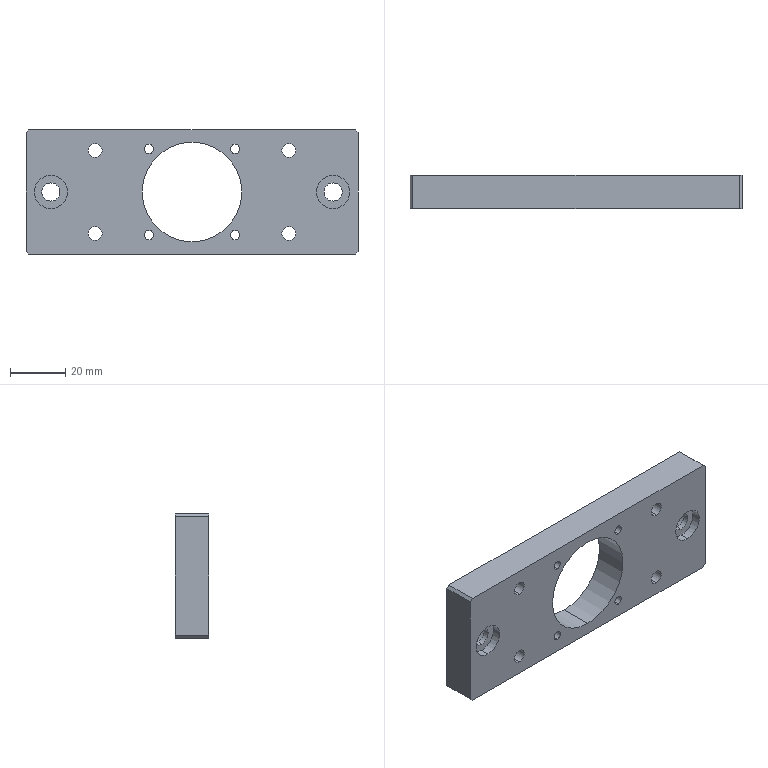Part | SolidWorks | features HoleWzd 4, ICE 2, Chamfer 1, Extrusion 1 | 1 solid | 48 faces | box 120 x 12 x 45 mm | volume 48954 mm3 | cylinder 32 | plane 14 | cone 2 | commonest cylinder face diameters 3.3 x10 5 x8 6.6 x4 11 x4 12 x4 36 x2
STEP:
#1=CARTESIAN_POINT('',(35.,0.,17.5));
#2=VERTEX_POINT('',#1);
#3=CARTESIAN_POINT('',(35.,0.,12.5));
#4=VERTEX_POINT('',#3);
#5=CARTESIAN_POINT('',(35.,0.,15.));
#6=DIRECTION('',(0.,-1.,0.));
#7=DIRECTION('',(0.,0.,-1.));
#8=AXIS2_PLACEMENT_3D('',#5,#6,#7);
#9=CIRCLE('',#8,2.5);
#10=EDGE_CURVE('',#2,#4,#9,.T.);
#11=ORIENTED_EDGE('',*,*,#10,.T.);
#12=CARTESIAN_POINT('',(35.,12.,12.5));
#13=VERTEX_POINT('',#12);
#14=CARTESIAN_POINT('',(35.,12.,12.5));
#15=DIRECTION('',(0.,1.,0.));
#16=VECTOR('',#15,1000.);
#17=LINE('',#14,#16);
#18=EDGE_CURVE('',#4,#13,#17,.T.);
#19=ORIENTED_EDGE('',*,*,#18,.T.);
#20=CARTESIAN_POINT('',(35.,12.,17.5));
#21=VERTEX_POINT('',#20);
#22=CARTESIAN_POINT('',(35.,12.,15.));
#23=DIRECTION('',(0.,1.,0.));
#24=DIRECTION('',(0.,0.,1.));
#25=AXIS2_PLACEMENT_3D('',#22,#23,#24);
#26=CIRCLE('',#25,2.5);
#27=EDGE_CURVE('',#13,#21,#26,.T.);
#28=ORIENTED_EDGE('',*,*,#27,.T.);
#29=CARTESIAN_POINT('',(35.,12.,17.5));
#30=DIRECTION('',(0.,1.,0.));
#31=VECTOR('',#30,1000.);
#32=LINE('',#29,#31);
#33=EDGE_CURVE('',#2,#21,#32,.T.);
#34=ORIENTED_EDGE('',*,*,#33,.F.);
#35=EDGE_LOOP('',(#11,#19,#28,#34));
#36=FACE_OUTER_BOUND('',#35,.T.);
#37=CARTESIAN_POINT('',(35.,12.,15.));
#38=DIRECTION('',(0.,1.,0.));
#39=DIRECTION('',(0.,0.,1.));
#40=AXIS2_PLACEMENT_3D('',#37,#38,#39);
#41=CYLINDRICAL_SURFACE('',#40,2.5);
#42=ADVANCED_FACE('',(#36),#41,.F.);
#43=CARTESIAN_POINT('',(35.,0.,-12.5));
#44=VERTEX_POINT('',#43);
#45=CARTESIAN_POINT('',(35.,0.,-17.5));
#46=VERTEX_POINT('',#45);
#47=CARTESIAN_POINT('',(35.,0.,-15.));
#48=DIRECTION('',(0.,-1.,0.));
#49=DIRECTION('',(0.,0.,-1.));
#50=AXIS2_PLACEMENT_3D('',#47,#48,#49);
#51=CIRCLE('',#50,2.5);
#52=EDGE_CURVE('',#44,#46,#51,.T.);
#53=ORIENTED_EDGE('',*,*,#52,.T.);
#54=CARTESIAN_POINT('',(35.,12.,-17.5));
#55=VERTEX_POINT('',#54);
#56=CARTESIAN_POINT('',(35.,12.,-17.5));
#57=DIRECTION('',(0.,1.,0.));
#58=VECTOR('',#57,1000.);
#59=LINE('',#56,#58);
#60=EDGE_CURVE('',#46,#55,#59,.T.);
#61=ORIENTED_EDGE('',*,*,#60,.T.);
#62=CARTESIAN_POINT('',(35.,12.,-12.5));
#63=VERTEX_POINT('',#62);
#64=CARTESIAN_POINT('',(35.,12.,-15.));
#65=DIRECTION('',(0.,1.,0.));
#66=DIRECTION('',(0.,0.,1.));
#67=AXIS2_PLACEMENT_3D('',#64,#65,#66);
#68=CIRCLE('',#67,2.5);
#69=EDGE_CURVE('',#55,#63,#68,.T.);
#70=ORIENTED_EDGE('',*,*,#69,.T.);
#71=CARTESIAN_POINT('',(35.,12.,-12.5));
#72=DIRECTION('',(0.,1.,0.));
#73=VECTOR('',#72,1000.);
#74=LINE('',#71,#73);
#75=EDGE_CURVE('',#44,#63,#74,.T.);
#76=ORIENTED_EDGE('',*,*,#75,.F.);
#77=EDGE_LOOP('',(#53,#61,#70,#76));
#78=FACE_OUTER_BOUND('',#77,.T.);
#79=CARTESIAN_POINT('',(35.,12.,-15.));
#80=DIRECTION('',(0.,1.,0.));
#81=DIRECTION('',(0.,0.,1.));
#82=AXIS2_PLACEMENT_3D('',#79,#80,#81);
#83=CYLINDRICAL_SURFACE('',#82,2.5);
#84=ADVANCED_FACE('',(#78),#83,.F.);
#85=CARTESIAN_POINT('',(-35.,0.,17.5));
#86=VERTEX_POINT('',#85);
#87=CARTESIAN_POINT('',(-35.,0.,12.5));
#88=VERTEX_POINT('',#87);
#89=CARTESIAN_POINT('',(-35.,0.,15.));
#90=DIRECTION('',(0.,-1.,0.));
#91=DIRECTION('',(0.,0.,-1.));
#92=AXIS2_PLACEMENT_3D('',#89,#90,#91);
#93=CIRCLE('',#92,2.5);
#94=EDGE_CURVE('',#86,#88,#93,.T.);
#95=ORIENTED_EDGE('',*,*,#94,.T.);
#96=CARTESIAN_POINT('',(-35.,12.,12.5));
#97=VERTEX_POINT('',#96);
#98=CARTESIAN_POINT('',(-35.,12.,12.5));
#99=DIRECTION('',(0.,1.,0.));
#100=VECTOR('',#99,1000.);
#101=LINE('',#98,#100);
#102=EDGE_CURVE('',#88,#97,#101,.T.);
#103=ORIENTED_EDGE('',*,*,#102,.T.);
#104=CARTESIAN_POINT('',(-35.,12.,17.5));
#105=VERTEX_POINT('',#104);
#106=CARTESIAN_POINT('',(-35.,12.,15.));
#107=DIRECTION('',(0.,1.,0.));
#108=DIRECTION('',(0.,0.,1.));
#109=AXIS2_PLACEMENT_3D('',#106,#107,#108);
#110=CIRCLE('',#109,2.5);
#111=EDGE_CURVE('',#97,#105,#110,.T.);
#112=ORIENTED_EDGE('',*,*,#111,.T.);
#113=CARTESIAN_POINT('',(-35.,12.,17.5));
#114=DIRECTION('',(0.,1.,0.));
#115=VECTOR('',#114,1000.);
#116=LINE('',#113,#115);
#117=EDGE_CURVE('',#86,#105,#116,.T.);
#118=ORIENTED_EDGE('',*,*,#117,.F.);
#119=EDGE_LOOP('',(#95,#103,#112,#118));
#120=FACE_OUTER_BOUND('',#119,.T.);
#121=CARTESIAN_POINT('',(-35.,12.,15.));
#122=DIRECTION('',(0.,1.,0.));
#123=DIRECTION('',(0.,0.,1.));
#124=AXIS2_PLACEMENT_3D('',#121,#122,#123);
#125=CYLINDRICAL_SURFACE('',#124,2.5);
#126=ADVANCED_FACE('',(#120),#125,.F.);
#127=CARTESIAN_POINT('',(-35.,0.,-12.5));
#128=VERTEX_POINT('',#127);
#129=CARTESIAN_POINT('',(-35.,0.,-17.5));
#130=VERTEX_POINT('',#129);
#131=CARTESIAN_POINT('',(-35.,0.,-15.));
#132=DIRECTION('',(0.,-1.,0.));
#133=DIRECTION('',(0.,0.,-1.));
#134=AXIS2_PLACEMENT_3D('',#131,#132,#133);
#135=CIRCLE('',#134,2.5);
#136=EDGE_CURVE('',#128,#130,#135,.T.);
#137=ORIENTED_EDGE('',*,*,#136,.T.);
#138=CARTESIAN_POINT('',(-35.,12.,-17.5));
#139=VERTEX_POINT('',#138);
#140=CARTESIAN_POINT('',(-35.,12.,-17.5));
#141=DIRECTION('',(0.,1.,0.));
#142=VECTOR('',#141,1000.);
#143=LINE('',#140,#142);
#144=EDGE_CURVE('',#130,#139,#143,.T.);
#145=ORIENTED_EDGE('',*,*,#144,.T.);
#146=CARTESIAN_POINT('',(-35.,12.,-12.5));
#147=VERTEX_POINT('',#146);
#148=CARTESIAN_POINT('',(-35.,12.,-15.));
#149=DIRECTION('',(0.,1.,0.));
#150=DIRECTION('',(0.,0.,1.));
#151=AXIS2_PLACEMENT_3D('',#148,#149,#150);
#152=CIRCLE('',#151,2.5);
#153=EDGE_CURVE('',#139,#147,#152,.T.);
#154=ORIENTED_EDGE('',*,*,#153,.T.);
#155=CARTESIAN_POINT('',(-35.,12.,-12.5));
#156=DIRECTION('',(0.,1.,0.));
#157=VECTOR('',#156,1000.);
#158=LINE('',#155,#157);
#159=EDGE_CURVE('',#128,#147,#158,.T.);
#160=ORIENTED_EDGE('',*,*,#159,.F.);
#161=EDGE_LOOP('',(#137,#145,#154,#160));
#162=FACE_OUTER_BOUND('',#161,.T.);
#163=CARTESIAN_POINT('',(-35.,12.,-15.));
#164=DIRECTION('',(0.,1.,0.));
#165=DIRECTION('',(0.,0.,1.));
#166=AXIS2_PLACEMENT_3D('',#163,#164,#165);
#167=CYLINDRICAL_SURFACE('',#166,2.5);
#168=ADVANCED_FACE('',(#162),#167,.F.);
#169=CARTESIAN_POINT('',(29.15,7.,-11.));
#170=VERTEX_POINT('',#169);
#171=CARTESIAN_POINT('',(25.85,7.,-11.));
#172=VERTEX_POINT('',#171);
#173=CARTESIAN_POINT('',(27.5,7.,-11.));
#174=DIRECTION('',(0.,0.,-1.));
#175=DIRECTION('',(-1.,0.,0.));
#176=AXIS2_PLACEMENT_3D('',#173,#174,#175);
#177=CIRCLE('',#176,1.65);
#178=EDGE_CURVE('',#170,#172,#177,.T.);
#179=ORIENTED_EDGE('',*,*,#178,.F.);
#180=CARTESIAN_POINT('',(29.15,7.,-22.5));
#181=VERTEX_POINT('',#180);
#182=CARTESIAN_POINT('',(29.15,7.,-22.5));
#183=DIRECTION('',(0.,0.,-1.));
#184=VECTOR('',#183,1000.);
#185=LINE('',#182,#184);
#186=EDGE_CURVE('',#170,#181,#185,.T.);
#187=ORIENTED_EDGE('',*,*,#186,.T.);
#188=CARTESIAN_POINT('',(25.85,7.,-22.5));
#189=VERTEX_POINT('',#188);
#190=CARTESIAN_POINT('',(27.5,7.,-22.5));
#191=DIRECTION('',(0.,0.,-1.));
#192=DIRECTION('',(-1.,0.,0.));
#193=AXIS2_PLACEMENT_3D('',#190,#191,#192);
#194=CIRCLE('',#193,1.65);
#195=EDGE_CURVE('',#181,#189,#194,.T.);
#196=ORIENTED_EDGE('',*,*,#195,.T.);
#197=CARTESIAN_POINT('',(25.85,7.,-22.5));
#198=DIRECTION('',(0.,0.,-1.));
#199=VECTOR('',#198,1000.);
#200=LINE('',#197,#199);
#201=EDGE_CURVE('',#172,#189,#200,.T.);
#202=ORIENTED_EDGE('',*,*,#201,.F.);
#203=EDGE_LOOP('',(#179,#187,#196,#202));
#204=FACE_OUTER_BOUND('',#203,.T.);
#205=CARTESIAN_POINT('',(27.5,7.,-22.5));
#206=DIRECTION('',(0.,0.,-1.));
#207=DIRECTION('',(-1.,0.,0.));
#208=AXIS2_PLACEMENT_3D('',#205,#206,#207);
#209=CYLINDRICAL_SURFACE('',#208,1.65);
#210=ADVANCED_FACE('',(#204),#209,.F.);
#211=CARTESIAN_POINT('',(27.5,7.,-10.009));
#212=VERTEX_POINT('',#211);
#213=CARTESIAN_POINT('',(25.85,7.,-11.));
#214=DIRECTION('',(-0.8572,0.,-0.515));
#215=VECTOR('',#214,1000.);
#216=LINE('',#213,#215);
#217=EDGE_CURVE('',#212,#172,#216,.T.);
#218=ORIENTED_EDGE('',*,*,#217,.F.);
#219=CARTESIAN_POINT('',(29.15,7.,-11.));
#220=DIRECTION('',(0.8572,0.,-0.515));
#221=VECTOR('',#220,1000.);
#222=LINE('',#219,#221);
#223=EDGE_CURVE('',#212,#170,#222,.T.);
#224=ORIENTED_EDGE('',*,*,#223,.T.);
#225=ORIENTED_EDGE('',*,*,#178,.T.);
#226=EDGE_LOOP('',(#218,#224,#225));
#227=FACE_OUTER_BOUND('',#226,.T.);
#228=CARTESIAN_POINT('',(27.5,7.,-11.));
#229=DIRECTION('',(0.,0.,-1.));
#230=DIRECTION('',(-1.,0.,0.));
#231=AXIS2_PLACEMENT_3D('',#228,#229,#230);
#232=CONICAL_SURFACE('',#231,1.65,1.03);
#233=ADVANCED_FACE('',(#227),#232,.F.);
#234=CARTESIAN_POINT('',(-51.,3.2,6.));
#235=VERTEX_POINT('',#234);
#236=CARTESIAN_POINT('',(-51.,3.2,-6.));
#237=VERTEX_POINT('',#236);
#238=CARTESIAN_POINT('',(-51.,3.2,0.));
#239=DIRECTION('',(0.,-1.,0.));
#240=DIRECTION('',(0.,0.,-1.));
#241=AXIS2_PLACEMENT_3D('',#238,#239,#240);
#242=CIRCLE('',#241,6.);
#243=EDGE_CURVE('',#235,#237,#242,.T.);
#244=ORIENTED_EDGE('',*,*,#243,.F.);
#245=CARTESIAN_POINT('',(-51.,0.,6.));
#246=VERTEX_POINT('',#245);
#247=CARTESIAN_POINT('',(-51.,3.2,6.));
#248=DIRECTION('',(0.,-1.,0.));
#249=VECTOR('',#248,1000.);
#250=LINE('',#247,#249);
#251=EDGE_CURVE('',#235,#246,#250,.T.);
#252=ORIENTED_EDGE('',*,*,#251,.T.);
#253=CARTESIAN_POINT('',(-51.,0.,-6.));
#254=VERTEX_POINT('',#253);
#255=CARTESIAN_POINT('',(-51.,0.,0.));
#256=DIRECTION('',(0.,-1.,0.));
#257=DIRECTION('',(0.,0.,-1.));
#258=AXIS2_PLACEMENT_3D('',#255,#256,#257);
#259=CIRCLE('',#258,6.);
#260=EDGE_CURVE('',#246,#254,#259,.T.);
#261=ORIENTED_EDGE('',*,*,#260,.T.);
#262=CARTESIAN_POINT('',(-51.,3.2,-6.));
#263=DIRECTION('',(0.,-1.,0.));
#264=VECTOR('',#263,1000.);
#265=LINE('',#262,#264);
#266=EDGE_CURVE('',#237,#254,#265,.T.);
#267=ORIENTED_EDGE('',*,*,#266,.F.);
#268=EDGE_LOOP('',(#244,#252,#261,#267));
#269=FACE_OUTER_BOUND('',#268,.T.);
#270=CARTESIAN_POINT('',(-51.,3.2,0.));
#271=DIRECTION('',(0.,-1.,0.));
#272=DIRECTION('',(0.,0.,-1.));
#273=AXIS2_PLACEMENT_3D('',#270,#271,#272);
#274=CYLINDRICAL_SURFACE('',#273,6.);
#275=ADVANCED_FACE('',(#269),#274,.F.);
#276=CARTESIAN_POINT('',(51.,3.2,6.));
#277=VERTEX_POINT('',#276);
#278=CARTESIAN_POINT('',(51.,3.2,-6.));
#279=VERTEX_POINT('',#278);
#280=CARTESIAN_POINT('',(51.,3.2,0.));
#281=DIRECTION('',(0.,-1.,0.));
#282=DIRECTION('',(0.,0.,-1.));
#283=AXIS2_PLACEMENT_3D('',#280,#281,#282);
#284=CIRCLE('',#283,6.);
#285=EDGE_CURVE('',#277,#279,#284,.T.);
#286=ORIENTED_EDGE('',*,*,#285,.F.);
#287=CARTESIAN_POINT('',(51.,0.,6.));
#288=VERTEX_POINT('',#287);
#289=CARTESIAN_POINT('',(51.,3.2,6.));
#290=DIRECTION('',(0.,-1.,0.));
#291=VECTOR('',#290,1000.);
#292=LINE('',#289,#291);
#293=EDGE_CURVE('',#277,#288,#292,.T.);
#294=ORIENTED_EDGE('',*,*,#293,.T.);
#295=CARTESIAN_POINT('',(51.,0.,-6.));
#296=VERTEX_POINT('',#295);
#297=CARTESIAN_POINT('',(51.,0.,0.));
#298=DIRECTION('',(0.,-1.,0.));
#299=DIRECTION('',(0.,0.,-1.));
#300=AXIS2_PLACEMENT_3D('',#297,#298,#299);
#301=CIRCLE('',#300,6.);
#302=EDGE_CURVE('',#288,#296,#301,.T.);
#303=ORIENTED_EDGE('',*,*,#302,.T.);
#304=CARTESIAN_POINT('',(51.,3.2,-6.));
#305=DIRECTION('',(0.,-1.,0.));
#306=VECTOR('',#305,1000.);
#307=LINE('',#304,#306);
#308=EDGE_CURVE('',#279,#296,#307,.T.);
#309=ORIENTED_EDGE('',*,*,#308,.F.);
#310=EDGE_LOOP('',(#286,#294,#303,#309));
#311=FACE_OUTER_BOUND('',#310,.T.);
#312=CARTESIAN_POINT('',(51.,3.2,0.));
#313=DIRECTION('',(0.,-1.,0.));
#314=DIRECTION('',(0.,0.,-1.));
#315=AXIS2_PLACEMENT_3D('',#312,#313,#314);
#316=CYLINDRICAL_SURFACE('',#315,6.);
#317=ADVANCED_FACE('',(#311),#316,.F.);
#318=CARTESIAN_POINT('',(-51.,5.2,-5.5));
#319=VERTEX_POINT('',#318);
#320=CARTESIAN_POINT('',(-51.,5.2,5.5));
#321=VERTEX_POINT('',#320);
#322=CARTESIAN_POINT('',(-51.,5.2,0.));
#323=DIRECTION('',(0.,1.,0.));
#324=DIRECTION('',(0.,0.,1.));
#325=AXIS2_PLACEMENT_3D('',#322,#323,#324);
#326=CIRCLE('',#325,5.5);
#327=EDGE_CURVE('',#319,#321,#326,.T.);
#328=ORIENTED_EDGE('',*,*,#327,.F.);
#329=CARTESIAN_POINT('',(-51.,12.,-5.5));
#330=VERTEX_POINT('',#329);
#331=CARTESIAN_POINT('',(-51.,12.,-5.5));
#332=DIRECTION('',(0.,1.,0.));
#333=VECTOR('',#332,1000.);
#334=LINE('',#331,#333);
#335=EDGE_CURVE('',#319,#330,#334,.T.);
#336=ORIENTED_EDGE('',*,*,#335,.T.);
#337=CARTESIAN_POINT('',(-51.,12.,5.5));
#338=VERTEX_POINT('',#337);
#339=CARTESIAN_POINT('',(-51.,12.,0.));
#340=DIRECTION('',(0.,1.,0.));
#341=DIRECTION('',(0.,0.,1.));
#342=AXIS2_PLACEMENT_3D('',#339,#340,#341);
#343=CIRCLE('',#342,5.5);
#344=EDGE_CURVE('',#330,#338,#343,.T.);
#345=ORIENTED_EDGE('',*,*,#344,.T.);
#346=CARTESIAN_POINT('',(-51.,12.,5.5));
#347=DIRECTION('',(0.,1.,0.));
#348=VECTOR('',#347,1000.);
#349=LINE('',#346,#348);
#350=EDGE_CURVE('',#321,#338,#349,.T.);
#351=ORIENTED_EDGE('',*,*,#350,.F.);
#352=EDGE_LOOP('',(#328,#336,#345,#351));
#353=FACE_OUTER_BOUND('',#352,.T.);
#354=CARTESIAN_POINT('',(-51.,12.,0.));
#355=DIRECTION('',(0.,1.,0.));
#356=DIRECTION('',(0.,0.,1.));
#357=AXIS2_PLACEMENT_3D('',#354,#355,#356);
#358=CYLINDRICAL_SURFACE('',#357,5.5);
#359=ADVANCED_FACE('',(#353),#358,.F.);
#360=CARTESIAN_POINT('',(51.,5.2,-5.5));
#361=VERTEX_POINT('',#360);
#362=CARTESIAN_POINT('',(51.,5.2,5.5));
#363=VERTEX_POINT('',#362);
#364=CARTESIAN_POINT('',(51.,5.2,0.));
#365=DIRECTION('',(0.,1.,0.));
#366=DIRECTION('',(0.,0.,1.));
#367=AXIS2_PLACEMENT_3D('',#364,#365,#366);
#368=CIRCLE('',#367,5.5);
#369=EDGE_CURVE('',#361,#363,#368,.T.);
#370=ORIENTED_EDGE('',*,*,#369,.F.);
#371=CARTESIAN_POINT('',(51.,12.,-5.5));
#372=VERTEX_POINT('',#371);
#373=CARTESIAN_POINT('',(51.,12.,-5.5));
#374=DIRECTION('',(0.,1.,0.));
#375=VECTOR('',#374,1000.);
#376=LINE('',#373,#375);
#377=EDGE_CURVE('',#361,#372,#376,.T.);
#378=ORIENTED_EDGE('',*,*,#377,.T.);
#379=CARTESIAN_POINT('',(51.,12.,5.5));
#380=VERTEX_POINT('',#379);
#381=CARTESIAN_POINT('',(51.,12.,0.));
#382=DIRECTION('',(0.,1.,0.));
#383=DIRECTION('',(0.,0.,1.));
#384=AXIS2_PLACEMENT_3D('',#381,#382,#383);
#385=CIRCLE('',#384,5.5);
#386=EDGE_CURVE('',#372,#380,#385,.T.);
#387=ORIENTED_EDGE('',*,*,#386,.T.);
#388=CARTESIAN_POINT('',(51.,12.,5.5));
#389=DIRECTION('',(0.,1.,0.));
#390=VECTOR('',#389,1000.);
#391=LINE('',#388,#390);
#392=EDGE_CURVE('',#363,#380,#391,.T.);
#393=ORIENTED_EDGE('',*,*,#392,.F.);
#394=EDGE_LOOP('',(#370,#378,#387,#393));
#395=FACE_OUTER_BOUND('',#394,.T.);
#396=CARTESIAN_POINT('',(51.,12.,0.));
#397=DIRECTION('',(0.,1.,0.));
#398=DIRECTION('',(0.,0.,1.));
#399=AXIS2_PLACEMENT_3D('',#396,#397,#398);
#400=CYLINDRICAL_SURFACE('',#399,5.5);
#401=ADVANCED_FACE('',(#395),#400,.F.);
#402=CARTESIAN_POINT('',(-15.556,0.,-17.206));
#403=VERTEX_POINT('',#402);
#404=CARTESIAN_POINT('',(-15.556,0.,-13.907));
#405=VERTEX_POINT('',#404);
#406=CARTESIAN_POINT('',(-15.556,0.,-15.556));
#407=DIRECTION('',(0.,1.,0.));
#408=DIRECTION('',(0.,0.,1.));
#409=AXIS2_PLACEMENT_3D('',#406,#407,#408);
#410=CIRCLE('',#409,1.65);
#411=EDGE_CURVE('',#403,#405,#410,.T.);
#412=ORIENTED_EDGE('',*,*,#411,.F.);
#413=CARTESIAN_POINT('',(-15.556,12.,-17.206));
#414=VERTEX_POINT('',#413);
#415=CARTESIAN_POINT('',(-15.556,12.,-17.206));
#416=DIRECTION('',(0.,1.,0.));
#417=VECTOR('',#416,1000.);
#418=LINE('',#415,#417);
#419=EDGE_CURVE('',#403,#414,#418,.T.);
#420=ORIENTED_EDGE('',*,*,#419,.T.);
#421=CARTESIAN_POINT('',(-15.556,12.,-13.907));
#422=VERTEX_POINT('',#421);
#423=CARTESIAN_POINT('',(-15.556,12.,-15.556));
#424=DIRECTION('',(0.,1.,0.));
#425=DIRECTION('',(0.,0.,1.));
#426=AXIS2_PLACEMENT_3D('',#423,#424,#425);
#427=CIRCLE('',#426,1.65);
#428=EDGE_CURVE('',#414,#422,#427,.T.);
#429=ORIENTED_EDGE('',*,*,#428,.T.);
#430=CARTESIAN_POINT('',(-15.556,12.,-13.907));
#431=DIRECTION('',(0.,1.,0.));
#432=VECTOR('',#431,1000.);
#433=LINE('',#430,#432);
#434=EDGE_CURVE('',#405,#422,#433,.T.);
#435=ORIENTED_EDGE('',*,*,#434,.F.);
#436=EDGE_LOOP('',(#412,#420,#429,#435));
#437=FACE_OUTER_BOUND('',#436,.T.);
#438=CARTESIAN_POINT('',(-15.556,12.,-15.556));
#439=DIRECTION('',(0.,1.,0.));
#440=DIRECTION('',(0.,0.,1.));
#441=AXIS2_PLACEMENT_3D('',#438,#439,#440);
#442=CYLINDRICAL_SURFACE('',#441,1.65);
#443=ADVANCED_FACE('',(#437),#442,.F.);
#444=CARTESIAN_POINT('',(-15.556,0.,13.907));
#445=VERTEX_POINT('',#444);
#446=CARTESIAN_POINT('',(-15.556,0.,17.206));
#447=VERTEX_POINT('',#446);
#448=CARTESIAN_POINT('',(-15.556,0.,15.556));
#449=DIRECTION('',(0.,1.,0.));
#450=DIRECTION('',(0.,0.,1.));
#451=AXIS2_PLACEMENT_3D('',#448,#449,#450);
#452=CIRCLE('',#451,1.65);
#453=EDGE_CURVE('',#445,#447,#452,.T.);
#454=ORIENTED_EDGE('',*,*,#453,.F.);
#455=CARTESIAN_POINT('',(-15.556,12.,13.907));
#456=VERTEX_POINT('',#455);
#457=CARTESIAN_POINT('',(-15.556,12.,13.907));
#458=DIRECTION('',(0.,1.,0.));
#459=VECTOR('',#458,1000.);
#460=LINE('',#457,#459);
#461=EDGE_CURVE('',#445,#456,#460,.T.);
#462=ORIENTED_EDGE('',*,*,#461,.T.);
#463=CARTESIAN_POINT('',(-15.556,12.,17.206));
#464=VERTEX_POINT('',#463);
#465=CARTESIAN_POINT('',(-15.556,12.,15.556));
#466=DIRECTION('',(0.,1.,0.));
#467=DIRECTION('',(0.,0.,1.));
#468=AXIS2_PLACEMENT_3D('',#465,#466,#467);
#469=CIRCLE('',#468,1.65);
#470=EDGE_CURVE('',#456,#464,#469,.T.);
#471=ORIENTED_EDGE('',*,*,#470,.T.);
#472=CARTESIAN_POINT('',(-15.556,12.,17.206));
#473=DIRECTION('',(0.,1.,0.));
#474=VECTOR('',#473,1000.);
#475=LINE('',#472,#474);
#476=EDGE_CURVE('',#447,#464,#475,.T.);
#477=ORIENTED_EDGE('',*,*,#476,.F.);
#478=EDGE_LOOP('',(#454,#462,#471,#477));
#479=FACE_OUTER_BOUND('',#478,.T.);
#480=CARTESIAN_POINT('',(-15.556,12.,15.556));
#481=DIRECTION('',(0.,1.,0.));
#482=DIRECTION('',(0.,0.,1.));
#483=AXIS2_PLACEMENT_3D('',#480,#481,#482);
#484=CYLINDRICAL_SURFACE('',#483,1.65);
#485=ADVANCED_FACE('',(#479),#484,.F.);
#486=CARTESIAN_POINT('',(15.556,0.,13.907));
#487=VERTEX_POINT('',#486);
#488=CARTESIAN_POINT('',(15.556,0.,17.206));
#489=VERTEX_POINT('',#488);
#490=CARTESIAN_POINT('',(15.556,0.,15.556));
#491=DIRECTION('',(0.,1.,0.));
#492=DIRECTION('',(0.,0.,1.));
#493=AXIS2_PLACEMENT_3D('',#490,#491,#492);
#494=CIRCLE('',#493,1.65);
#495=EDGE_CURVE('',#487,#489,#494,.T.);
#496=ORIENTED_EDGE('',*,*,#495,.F.);
#497=CARTESIAN_POINT('',(15.556,12.,13.907));
#498=VERTEX_POINT('',#497);
#499=CARTESIAN_POINT('',(15.556,12.,13.907));
#500=DIRECTION('',(0.,1.,0.));
#501=VECTOR('',#500,1000.);
#502=LINE('',#499,#501);
#503=EDGE_CURVE('',#487,#498,#502,.T.);
#504=ORIENTED_EDGE('',*,*,#503,.T.);
#505=CARTESIAN_POINT('',(15.556,12.,17.206));
#506=VERTEX_POINT('',#505);
#507=CARTESIAN_POINT('',(15.556,12.,15.556));
#508=DIRECTION('',(0.,1.,0.));
#509=DIRECTION('',(0.,0.,1.));
#510=AXIS2_PLACEMENT_3D('',#507,#508,#509);
#511=CIRCLE('',#510,1.65);
#512=EDGE_CURVE('',#498,#506,#511,.T.);
#513=ORIENTED_EDGE('',*,*,#512,.T.);
#514=CARTESIAN_POINT('',(15.556,12.,17.206));
#515=DIRECTION('',(0.,1.,0.));
#516=VECTOR('',#515,1000.);
#517=LINE('',#514,#516);
#518=EDGE_CURVE('',#489,#506,#517,.T.);
#519=ORIENTED_EDGE('',*,*,#518,.F.);
#520=EDGE_LOOP('',(#496,#504,#513,#519));
#521=FACE_OUTER_BOUND('',#520,.T.);
#522=CARTESIAN_POINT('',(15.556,12.,15.556));
#523=DIRECTION('',(0.,1.,0.));
#524=DIRECTION('',(0.,0.,1.));
#525=AXIS2_PLACEMENT_3D('',#522,#523,#524);
#526=CYLINDRICAL_SURFACE('',#525,1.65);
#527=ADVANCED_FACE('',(#521),#526,.F.);
#528=CARTESIAN_POINT('',(15.556,0.,-17.206));
#529=VERTEX_POINT('',#528);
#530=CARTESIAN_POINT('',(15.556,0.,-13.907));
#531=VERTEX_POINT('',#530);
#532=CARTESIAN_POINT('',(15.556,0.,-15.556));
#533=DIRECTION('',(0.,1.,0.));
#534=DIRECTION('',(0.,0.,1.));
#535=AXIS2_PLACEMENT_3D('',#532,#533,#534);
#536=CIRCLE('',#535,1.65);
#537=EDGE_CURVE('',#529,#531,#536,.T.);
#538=ORIENTED_EDGE('',*,*,#537,.F.);
#539=CARTESIAN_POINT('',(15.556,12.,-17.206));
#540=VERTEX_POINT('',#539);
#541=CARTESIAN_POINT('',(15.556,12.,-17.206));
#542=DIRECTION('',(0.,1.,0.));
#543=VECTOR('',#542,1000.);
#544=LINE('',#541,#543);
#545=EDGE_CURVE('',#529,#540,#544,.T.);
#546=ORIENTED_EDGE('',*,*,#545,.T.);
#547=CARTESIAN_POINT('',(15.556,12.,-13.907));
#548=VERTEX_POINT('',#547);
#549=CARTESIAN_POINT('',(15.556,12.,-15.556));
#550=DIRECTION('',(0.,1.,0.));
#551=DIRECTION('',(0.,0.,1.));
#552=AXIS2_PLACEMENT_3D('',#549,#550,#551);
#553=CIRCLE('',#552,1.65);
#554=EDGE_CURVE('',#540,#548,#553,.T.);
#555=ORIENTED_EDGE('',*,*,#554,.T.);
#556=CARTESIAN_POINT('',(15.556,12.,-13.907));
#557=DIRECTION('',(0.,1.,0.));
#558=VECTOR('',#557,1000.);
#559=LINE('',#556,#558);
#560=EDGE_CURVE('',#531,#548,#559,.T.);
#561=ORIENTED_EDGE('',*,*,#560,.F.);
#562=EDGE_LOOP('',(#538,#546,#555,#561));
#563=FACE_OUTER_BOUND('',#562,.T.);
#564=CARTESIAN_POINT('',(15.556,12.,-15.556));
#565=DIRECTION('',(0.,1.,0.));
#566=DIRECTION('',(0.,0.,1.));
#567=AXIS2_PLACEMENT_3D('',#564,#565,#566);
#568=CYLINDRICAL_SURFACE('',#567,1.65);
#569=ADVANCED_FACE('',(#563),#568,.F.);
#570=CARTESIAN_POINT('',(0.,0.,-18.));
#571=VERTEX_POINT('',#570);
#572=CARTESIAN_POINT('',(0.,0.,18.));
#573=VERTEX_POINT('',#572);
#574=CARTESIAN_POINT('',(0.,0.,0.));
#575=DIRECTION('',(0.,1.,0.));
#576=DIRECTION('',(0.,0.,1.));
#577=AXIS2_PLACEMENT_3D('',#574,#575,#576);
#578=CIRCLE('',#577,18.);
#579=EDGE_CURVE('',#571,#573,#578,.T.);
#580=ORIENTED_EDGE('',*,*,#579,.F.);
#581=CARTESIAN_POINT('',(0.,12.,-18.));
#582=VERTEX_POINT('',#581);
#583=CARTESIAN_POINT('',(0.,0.,-18.));
#584=DIRECTION('',(0.,1.,0.));
#585=VECTOR('',#584,1000.);
#586=LINE('',#583,#585);
#587=EDGE_CURVE('',#571,#582,#586,.T.);
#588=ORIENTED_EDGE('',*,*,#587,.T.);
#589=CARTESIAN_POINT('',(0.,12.,18.));
#590=VERTEX_POINT('',#589);
#591=CARTESIAN_POINT('',(0.,12.,0.));
#592=DIRECTION('',(0.,1.,0.));
#593=DIRECTION('',(0.,0.,1.));
#594=AXIS2_PLACEMENT_3D('',#591,#592,#593);
#595=CIRCLE('',#594,18.);
#596=EDGE_CURVE('',#582,#590,#595,.T.);
#597=ORIENTED_EDGE('',*,*,#596,.T.);
#598=CARTESIAN_POINT('',(0.,0.,18.));
#599=DIRECTION('',(0.,1.,0.));
#600=VECTOR('',#599,1000.);
#601=LINE('',#598,#600);
#602=EDGE_CURVE('',#573,#590,#601,.T.);
#603=ORIENTED_EDGE('',*,*,#602,.F.);
#604=EDGE_LOOP('',(#580,#588,#597,#603));
#605=FACE_OUTER_BOUND('',#604,.T.);
#606=CARTESIAN_POINT('',(0.,0.,0.));
#607=DIRECTION('',(0.,1.,0.));
#608=DIRECTION('',(0.,0.,1.));
#609=AXIS2_PLACEMENT_3D('',#606,#607,#608);
#610=CYLINDRICAL_SURFACE('',#609,18.);
#611=ADVANCED_FACE('',(#605),#610,.F.);
#612=CARTESIAN_POINT('',(51.,3.2,-3.3));
#613=VERTEX_POINT('',#612);
#614=CARTESIAN_POINT('',(51.,3.2,3.3));
#615=VERTEX_POINT('',#614);
#616=CARTESIAN_POINT('',(51.,3.2,0.));
#617=DIRECTION('',(0.,1.,0.));
#618=DIRECTION('',(0.,0.,-1.));
#619=AXIS2_PLACEMENT_3D('',#616,#617,#618);
#620=CIRCLE('',#619,3.3);
#621=EDGE_CURVE('',#613,#615,#620,.T.);
#622=ORIENTED_EDGE('',*,*,#621,.F.);
#623=CARTESIAN_POINT('',(51.,5.2,-3.3));
#624=VERTEX_POINT('',#623);
#625=CARTESIAN_POINT('',(51.,12.,-3.3));
#626=DIRECTION('',(0.,1.,0.));
#627=VECTOR('',#626,1000.);
#628=LINE('',#625,#627);
#629=EDGE_CURVE('',#613,#624,#628,.T.);
#630=ORIENTED_EDGE('',*,*,#629,.T.);
#631=CARTESIAN_POINT('',(51.,5.2,3.3));
#632=VERTEX_POINT('',#631);
#633=CARTESIAN_POINT('',(51.,5.2,0.));
#634=DIRECTION('',(0.,1.,0.));
#635=DIRECTION('',(0.,0.,1.));
#636=AXIS2_PLACEMENT_3D('',#633,#634,#635);
#637=CIRCLE('',#636,3.3);
#638=EDGE_CURVE('',#624,#632,#637,.T.);
#639=ORIENTED_EDGE('',*,*,#638,.T.);
#640=CARTESIAN_POINT('',(51.,12.,3.3));
#641=DIRECTION('',(0.,1.,0.));
#642=VECTOR('',#641,1000.);
#643=LINE('',#640,#642);
#644=EDGE_CURVE('',#615,#632,#643,.T.);
#645=ORIENTED_EDGE('',*,*,#644,.F.);
#646=EDGE_LOOP('',(#622,#630,#639,#645));
#647=FACE_OUTER_BOUND('',#646,.T.);
#648=CARTESIAN_POINT('',(51.,12.,0.));
#649=DIRECTION('',(0.,1.,0.));
#650=DIRECTION('',(0.,0.,1.));
#651=AXIS2_PLACEMENT_3D('',#648,#649,#650);
#652=CYLINDRICAL_SURFACE('',#651,3.3);
#653=ADVANCED_FACE('',(#647),#652,.F.);
#654=CARTESIAN_POINT('',(-51.,3.2,-3.3));
#655=VERTEX_POINT('',#654);
#656=CARTESIAN_POINT('',(-51.,3.2,3.3));
#657=VERTEX_POINT('',#656);
#658=CARTESIAN_POINT('',(-51.,3.2,0.));
#659=DIRECTION('',(0.,1.,0.));
#660=DIRECTION('',(0.,0.,-1.));
#661=AXIS2_PLACEMENT_3D('',#658,#659,#660);
#662=CIRCLE('',#661,3.3);
#663=EDGE_CURVE('',#655,#657,#662,.T.);
#664=ORIENTED_EDGE('',*,*,#663,.F.);
#665=CARTESIAN_POINT('',(-51.,5.2,-3.3));
#666=VERTEX_POINT('',#665);
#667=CARTESIAN_POINT('',(-51.,12.,-3.3));
#668=DIRECTION('',(0.,1.,0.));
#669=VECTOR('',#668,1000.);
#670=LINE('',#667,#669);
#671=EDGE_CURVE('',#655,#666,#670,.T.);
#672=ORIENTED_EDGE('',*,*,#671,.T.);
#673=CARTESIAN_POINT('',(-51.,5.2,3.3));
#674=VERTEX_POINT('',#673);
#675=CARTESIAN_POINT('',(-51.,5.2,0.));
#676=DIRECTION('',(0.,1.,0.));
#677=DIRECTION('',(0.,0.,1.));
#678=AXIS2_PLACEMENT_3D('',#675,#676,#677);
#679=CIRCLE('',#678,3.3);
#680=EDGE_CURVE('',#666,#674,#679,.T.);
#681=ORIENTED_EDGE('',*,*,#680,.T.);
#682=CARTESIAN_POINT('',(-51.,12.,3.3));
#683=DIRECTION('',(0.,1.,0.));
#684=VECTOR('',#683,1000.);
#685=LINE('',#682,#684);
#686=EDGE_CURVE('',#657,#674,#685,.T.);
#687=ORIENTED_EDGE('',*,*,#686,.F.);
#688=EDGE_LOOP('',(#664,#672,#681,#687));
#689=FACE_OUTER_BOUND('',#688,.T.);
#690=CARTESIAN_POINT('',(-51.,12.,0.));
#691=DIRECTION('',(0.,1.,0.));
#692=DIRECTION('',(0.,0.,1.));
#693=AXIS2_PLACEMENT_3D('',#690,#691,#692);
#694=CYLINDRICAL_SURFACE('',#693,3.3);
#695=ADVANCED_FACE('',(#689),#694,.F.);
#696=CARTESIAN_POINT('',(35.,12.,15.));
#697=DIRECTION('',(0.,1.,0.));
#698=DIRECTION('',(0.,0.,1.));
#699=AXIS2_PLACEMENT_3D('',#696,#697,#698);
#700=CIRCLE('',#699,2.5);
#701=EDGE_CURVE('',#21,#13,#700,.T.);
#702=ORIENTED_EDGE('',*,*,#701,.F.);
#703=ORIENTED_EDGE('',*,*,#27,.F.);
#704=EDGE_LOOP('',(#702,#703));
#705=FACE_BOUND('',#704,.T.);
#706=CARTESIAN_POINT('',(-35.,12.,-15.));
#707=DIRECTION('',(0.,1.,0.));
#708=DIRECTION('',(0.,0.,1.));
#709=AXIS2_PLACEMENT_3D('',#706,#707,#708);
#710=CIRCLE('',#709,2.5);
#711=EDGE_CURVE('',#147,#139,#710,.T.);
#712=ORIENTED_EDGE('',*,*,#711,.F.);
#713=ORIENTED_EDGE('',*,*,#153,.F.);
#714=EDGE_LOOP('',(#712,#713));
#715=FACE_BOUND('',#714,.T.);
#716=CARTESIAN_POINT('',(-15.556,12.,-15.556));
#717=DIRECTION('',(0.,1.,0.));
#718=DIRECTION('',(0.,0.,1.));
#719=AXIS2_PLACEMENT_3D('',#716,#717,#718);
#720=CIRCLE('',#719,1.65);
#721=EDGE_CURVE('',#422,#414,#720,.T.);
#722=ORIENTED_EDGE('',*,*,#721,.F.);
#723=ORIENTED_EDGE('',*,*,#428,.F.);
#724=EDGE_LOOP('',(#722,#723));
#725=FACE_BOUND('',#724,.T.);
#726=CARTESIAN_POINT('',(15.556,12.,15.556));
#727=DIRECTION('',(0.,1.,0.));
#728=DIRECTION('',(0.,0.,1.));
#729=AXIS2_PLACEMENT_3D('',#726,#727,#728);
#730=CIRCLE('',#729,1.65);
#731=EDGE_CURVE('',#506,#498,#730,.T.);
#732=ORIENTED_EDGE('',*,*,#731,.F.);
#733=ORIENTED_EDGE('',*,*,#512,.F.);
#734=EDGE_LOOP('',(#732,#733));
#735=FACE_BOUND('',#734,.T.);
#736=CARTESIAN_POINT('',(15.556,12.,-15.556));
#737=DIRECTION('',(0.,1.,0.));
#738=DIRECTION('',(0.,0.,1.));
#739=AXIS2_PLACEMENT_3D('',#736,#737,#738);
#740=CIRCLE('',#739,1.65);
#741=EDGE_CURVE('',#548,#540,#740,.T.);
#742=ORIENTED_EDGE('',*,*,#741,.F.);
#743=ORIENTED_EDGE('',*,*,#554,.F.);
#744=EDGE_LOOP('',(#742,#743));
#745=FACE_BOUND('',#744,.T.);
#746=CARTESIAN_POINT('',(0.,12.,0.));
#747=DIRECTION('',(0.,1.,0.));
#748=DIRECTION('',(0.,0.,1.));
#749=AXIS2_PLACEMENT_3D('',#746,#747,#748);
#750=CIRCLE('',#749,18.);
#751=EDGE_CURVE('',#590,#582,#750,.T.);
#752=ORIENTED_EDGE('',*,*,#751,.F.);
#753=ORIENTED_EDGE('',*,*,#596,.F.);
#754=EDGE_LOOP('',(#752,#753));
#755=FACE_BOUND('',#754,.T.);
#756=CARTESIAN_POINT('',(60.,12.,21.5));
#757=VERTEX_POINT('',#756);
#758=CARTESIAN_POINT('',(60.,12.,-21.5));
#759=VERTEX_POINT('',#758);
#760=CARTESIAN_POINT('',(60.,12.,-22.5));
#761=DIRECTION('',(0.,0.,-1.));
#762=VECTOR('',#761,1000.);
#763=LINE('',#760,#762);
#764=EDGE_CURVE('',#757,#759,#763,.T.);
#765=ORIENTED_EDGE('',*,*,#764,.T.);
#766=CARTESIAN_POINT('',(59.,12.,-22.5));
#767=VERTEX_POINT('',#766);
#768=CARTESIAN_POINT('',(59.,12.,-22.5));
#769=DIRECTION('',(-0.7071,0.,-0.7071));
#770=VECTOR('',#769,1000.);
#771=LINE('',#768,#770);
#772=EDGE_CURVE('',#759,#767,#771,.T.);
#773=ORIENTED_EDGE('',*,*,#772,.T.);
#774=CARTESIAN_POINT('',(-59.,12.,-22.5));
#775=VERTEX_POINT('',#774);
#776=CARTESIAN_POINT('',(60.,12.,-22.5));
#777=DIRECTION('',(-1.,0.,0.));
#778=VECTOR('',#777,1000.);
#779=LINE('',#776,#778);
#780=EDGE_CURVE('',#767,#775,#779,.T.);
#781=ORIENTED_EDGE('',*,*,#780,.T.);
#782=CARTESIAN_POINT('',(-60.,12.,-21.5));
#783=VERTEX_POINT('',#782);
#784=CARTESIAN_POINT('',(-60.,12.,-21.5));
#785=DIRECTION('',(-0.7071,0.,0.7071));
#786=VECTOR('',#785,1000.);
#787=LINE('',#784,#786);
#788=EDGE_CURVE('',#775,#783,#787,.T.);
#789=ORIENTED_EDGE('',*,*,#788,.T.);
#790=CARTESIAN_POINT('',(-60.,12.,21.5));
#791=VERTEX_POINT('',#790);
#792=CARTESIAN_POINT('',(-60.,12.,-22.5));
#793=DIRECTION('',(0.,0.,1.));
#794=VECTOR('',#793,1000.);
#795=LINE('',#792,#794);
#796=EDGE_CURVE('',#783,#791,#795,.T.);
#797=ORIENTED_EDGE('',*,*,#796,.T.);
#798=CARTESIAN_POINT('',(-59.,12.,22.5));
#799=VERTEX_POINT('',#798);
#800=CARTESIAN_POINT('',(-59.,12.,22.5));
#801=DIRECTION('',(0.7071,0.,0.7071));
#802=VECTOR('',#801,1000.);
#803=LINE('',#800,#802);
#804=EDGE_CURVE('',#791,#799,#803,.T.);
#805=ORIENTED_EDGE('',*,*,#804,.T.);
#806=CARTESIAN_POINT('',(59.,12.,22.5));
#807=VERTEX_POINT('',#806);
#808=CARTESIAN_POINT('',(60.,12.,22.5));
#809=DIRECTION('',(1.,0.,0.));
#810=VECTOR('',#809,1000.);
#811=LINE('',#808,#810);
#812=EDGE_CURVE('',#799,#807,#811,.T.);
#813=ORIENTED_EDGE('',*,*,#812,.T.);
#814=CARTESIAN_POINT('',(60.,12.,21.5));
#815=DIRECTION('',(0.7071,0.,-0.7071));
#816=VECTOR('',#815,1000.);
#817=LINE('',#814,#816);
#818=EDGE_CURVE('',#807,#757,#817,.T.);
#819=ORIENTED_EDGE('',*,*,#818,.T.);
#820=EDGE_LOOP('',(#765,#773,#781,#789,#797,#805,#813,#819));
#821=FACE_OUTER_BOUND('',#820,.T.);
#822=CARTESIAN_POINT('',(-15.556,12.,15.556));
#823=DIRECTION('',(0.,1.,0.));
#824=DIRECTION('',(0.,0.,1.));
#825=AXIS2_PLACEMENT_3D('',#822,#823,#824);
#826=CIRCLE('',#825,1.65);
#827=EDGE_CURVE('',#464,#456,#826,.T.);
#828=ORIENTED_EDGE('',*,*,#827,.F.);
#829=ORIENTED_EDGE('',*,*,#470,.F.);
#830=EDGE_LOOP('',(#828,#829));
#831=FACE_BOUND('',#830,.T.);
#832=CARTESIAN_POINT('',(51.,12.,0.));
#833=DIRECTION('',(0.,1.,0.));
#834=DIRECTION('',(0.,0.,1.));
#835=AXIS2_PLACEMENT_3D('',#832,#833,#834);
#836=CIRCLE('',#835,5.5);
#837=EDGE_CURVE('',#380,#372,#836,.T.);
#838=ORIENTED_EDGE('',*,*,#837,.F.);
#839=ORIENTED_EDGE('',*,*,#386,.F.);
#840=EDGE_LOOP('',(#838,#839));
#841=FACE_BOUND('',#840,.T.);
#842=CARTESIAN_POINT('',(-51.,12.,0.));
#843=DIRECTION('',(0.,1.,0.));
#844=DIRECTION('',(0.,0.,1.));
#845=AXIS2_PLACEMENT_3D('',#842,#843,#844);
#846=CIRCLE('',#845,5.5);
#847=EDGE_CURVE('',#338,#330,#846,.T.);
#848=ORIENTED_EDGE('',*,*,#847,.F.);
#849=ORIENTED_EDGE('',*,*,#344,.F.);
#850=EDGE_LOOP('',(#848,#849));
#851=FACE_BOUND('',#850,.T.);
#852=CARTESIAN_POINT('',(-35.,12.,15.));
#853=DIRECTION('',(0.,1.,0.));
#854=DIRECTION('',(0.,0.,1.));
#855=AXIS2_PLACEMENT_3D('',#852,#853,#854);
#856=CIRCLE('',#855,2.5);
#857=EDGE_CURVE('',#105,#97,#856,.T.);
#858=ORIENTED_EDGE('',*,*,#857,.F.);
#859=ORIENTED_EDGE('',*,*,#111,.F.);
#860=EDGE_LOOP('',(#858,#859));
#861=FACE_BOUND('',#860,.T.);
#862=CARTESIAN_POINT('',(35.,12.,-15.));
#863=DIRECTION('',(0.,1.,0.));
#864=DIRECTION('',(0.,0.,1.));
#865=AXIS2_PLACEMENT_3D('',#862,#863,#864);
#866=CIRCLE('',#865,2.5);
#867=EDGE_CURVE('',#63,#55,#866,.T.);
#868=ORIENTED_EDGE('',*,*,#867,.F.);
#869=ORIENTED_EDGE('',*,*,#69,.F.);
#870=EDGE_LOOP('',(#868,#869));
#871=FACE_BOUND('',#870,.T.);
#872=CARTESIAN_POINT('',(-60.,12.,22.5));
#873=DIRECTION('',(0.,-1.,0.));
#874=DIRECTION('',(0.,0.,-1.));
#875=AXIS2_PLACEMENT_3D('',#872,#873,#874);
#876=PLANE('',#875);
#877=ADVANCED_FACE('',(#705,#715,#725,#735,#745,#755,#821,#831,#841,#851,#861,#871),#876,.F.);
#878=ORIENTED_EDGE('',*,*,#671,.F.);
#879=CARTESIAN_POINT('',(-51.,3.2,0.));
#880=DIRECTION('',(0.,1.,0.));
#881=DIRECTION('',(0.,0.,-1.));
#882=AXIS2_PLACEMENT_3D('',#879,#880,#881);
#883=CIRCLE('',#882,3.3);
#884=EDGE_CURVE('',#657,#655,#883,.T.);
#885=ORIENTED_EDGE('',*,*,#884,.F.);
#886=ORIENTED_EDGE('',*,*,#686,.T.);
#887=CARTESIAN_POINT('',(-51.,5.2,0.));
#888=DIRECTION('',(0.,1.,0.));
#889=DIRECTION('',(0.,0.,1.));
#890=AXIS2_PLACEMENT_3D('',#887,#888,#889);
#891=CIRCLE('',#890,3.3);
#892=EDGE_CURVE('',#674,#666,#891,.T.);
#893=ORIENTED_EDGE('',*,*,#892,.T.);
#894=EDGE_LOOP('',(#878,#885,#886,#893));
#895=FACE_OUTER_BOUND('',#894,.T.);
#896=CARTESIAN_POINT('',(-51.,12.,0.));
#897=DIRECTION('',(0.,1.,0.));
#898=DIRECTION('',(0.,0.,1.));
#899=AXIS2_PLACEMENT_3D('',#896,#897,#898);
#900=CYLINDRICAL_SURFACE('',#899,3.3);
#901=ADVANCED_FACE('',(#895),#900,.F.);
#902=ORIENTED_EDGE('',*,*,#629,.F.);
#903=CARTESIAN_POINT('',(51.,3.2,0.));
#904=DIRECTION('',(0.,1.,0.));
#905=DIRECTION('',(0.,0.,-1.));
#906=AXIS2_PLACEMENT_3D('',#903,#904,#905);
#907=CIRCLE('',#906,3.3);
#908=EDGE_CURVE('',#615,#613,#907,.T.);
#909=ORIENTED_EDGE('',*,*,#908,.F.);
#910=ORIENTED_EDGE('',*,*,#644,.T.);
#911=CARTESIAN_POINT('',(51.,5.2,0.));
#912=DIRECTION('',(0.,1.,0.));
#913=DIRECTION('',(0.,0.,1.));
#914=AXIS2_PLACEMENT_3D('',#911,#912,#913);
#915=CIRCLE('',#914,3.3);
#916=EDGE_CURVE('',#632,#624,#915,.T.);
#917=ORIENTED_EDGE('',*,*,#916,.T.);
#918=EDGE_LOOP('',(#902,#909,#910,#917));
#919=FACE_OUTER_BOUND('',#918,.T.);
#920=CARTESIAN_POINT('',(51.,12.,0.));
#921=DIRECTION('',(0.,1.,0.));
#922=DIRECTION('',(0.,0.,1.));
#923=AXIS2_PLACEMENT_3D('',#920,#921,#922);
#924=CYLINDRICAL_SURFACE('',#923,3.3);
#925=ADVANCED_FACE('',(#919),#924,.F.);
#926=ORIENTED_EDGE('',*,*,#10,.F.);
#927=CARTESIAN_POINT('',(35.,0.,15.));
#928=DIRECTION('',(0.,-1.,0.));
#929=DIRECTION('',(0.,0.,-1.));
#930=AXIS2_PLACEMENT_3D('',#927,#928,#929);
#931=CIRCLE('',#930,2.5);
#932=EDGE_CURVE('',#4,#2,#931,.T.);
#933=ORIENTED_EDGE('',*,*,#932,.F.);
#934=EDGE_LOOP('',(#926,#933));
#935=FACE_BOUND('',#934,.T.);
#936=ORIENTED_EDGE('',*,*,#52,.F.);
#937=CARTESIAN_POINT('',(35.,0.,-15.));
#938=DIRECTION('',(0.,-1.,0.));
#939=DIRECTION('',(0.,0.,-1.));
#940=AXIS2_PLACEMENT_3D('',#937,#938,#939);
#941=CIRCLE('',#940,2.5);
#942=EDGE_CURVE('',#46,#44,#941,.T.);
#943=ORIENTED_EDGE('',*,*,#942,.F.);
#944=EDGE_LOOP('',(#936,#943));
#945=FACE_BOUND('',#944,.T.);
#946=ORIENTED_EDGE('',*,*,#94,.F.);
#947=CARTESIAN_POINT('',(-35.,0.,15.));
#948=DIRECTION('',(0.,-1.,0.));
#949=DIRECTION('',(0.,0.,-1.));
#950=AXIS2_PLACEMENT_3D('',#947,#948,#949);
#951=CIRCLE('',#950,2.5);
#952=EDGE_CURVE('',#88,#86,#951,.T.);
#953=ORIENTED_EDGE('',*,*,#952,.F.);
#954=EDGE_LOOP('',(#946,#953));
#955=FACE_BOUND('',#954,.T.);
#956=ORIENTED_EDGE('',*,*,#136,.F.);
#957=CARTESIAN_POINT('',(-35.,0.,-15.));
#958=DIRECTION('',(0.,-1.,0.));
#959=DIRECTION('',(0.,0.,-1.));
#960=AXIS2_PLACEMENT_3D('',#957,#958,#959);
#961=CIRCLE('',#960,2.5);
#962=EDGE_CURVE('',#130,#128,#961,.T.);
#963=ORIENTED_EDGE('',*,*,#962,.F.);
#964=EDGE_LOOP('',(#956,#963));
#965=FACE_BOUND('',#964,.T.);
#966=CARTESIAN_POINT('',(-51.,0.,0.));
#967=DIRECTION('',(0.,-1.,0.));
#968=DIRECTION('',(0.,0.,-1.));
#969=AXIS2_PLACEMENT_3D('',#966,#967,#968);
#970=CIRCLE('',#969,6.);
#971=EDGE_CURVE('',#254,#246,#970,.T.);
#972=ORIENTED_EDGE('',*,*,#971,.F.);
#973=ORIENTED_EDGE('',*,*,#260,.F.);
#974=EDGE_LOOP('',(#972,#973));
#975=FACE_BOUND('',#974,.T.);
#976=CARTESIAN_POINT('',(51.,0.,0.));
#977=DIRECTION('',(0.,-1.,0.));
#978=DIRECTION('',(0.,0.,-1.));
#979=AXIS2_PLACEMENT_3D('',#976,#977,#978);
#980=CIRCLE('',#979,6.);
#981=EDGE_CURVE('',#296,#288,#980,.T.);
#982=ORIENTED_EDGE('',*,*,#981,.F.);
#983=ORIENTED_EDGE('',*,*,#302,.F.);
#984=EDGE_LOOP('',(#982,#983));
#985=FACE_BOUND('',#984,.T.);
#986=CARTESIAN_POINT('',(-15.556,0.,-15.556));
#987=DIRECTION('',(0.,1.,0.));
#988=DIRECTION('',(0.,0.,1.));
#989=AXIS2_PLACEMENT_3D('',#986,#987,#988);
#990=CIRCLE('',#989,1.65);
#991=EDGE_CURVE('',#405,#403,#990,.T.);
#992=ORIENTED_EDGE('',*,*,#991,.T.);
#993=ORIENTED_EDGE('',*,*,#411,.T.);
#994=EDGE_LOOP('',(#992,#993));
#995=FACE_BOUND('',#994,.T.);
#996=CARTESIAN_POINT('',(15.556,0.,15.556));
#997=DIRECTION('',(0.,1.,0.));
#998=DIRECTION('',(0.,0.,1.));
#999=AXIS2_PLACEMENT_3D('',#996,#997,#998);
#1000=CIRCLE('',#999,1.65);
#1001=EDGE_CURVE('',#489,#487,#1000,.T.);
#1002=ORIENTED_EDGE('',*,*,#1001,.T.);
#1003=ORIENTED_EDGE('',*,*,#495,.T.);
#1004=EDGE_LOOP('',(#1002,#1003));
#1005=FACE_BOUND('',#1004,.T.);
#1006=CARTESIAN_POINT('',(15.556,0.,-15.556));
#1007=DIRECTION('',(0.,1.,0.));
#1008=DIRECTION('',(0.,0.,1.));
#1009=AXIS2_PLACEMENT_3D('',#1006,#1007,#1008);
#1010=CIRCLE('',#1009,1.65);
#1011=EDGE_CURVE('',#531,#529,#1010,.T.);
#1012=ORIENTED_EDGE('',*,*,#1011,.T.);
#1013=ORIENTED_EDGE('',*,*,#537,.T.);
#1014=EDGE_LOOP('',(#1012,#1013));
#1015=FACE_BOUND('',#1014,.T.);
#1016=CARTESIAN_POINT('',(0.,0.,0.));
#1017=DIRECTION('',(0.,1.,0.));
#1018=DIRECTION('',(0.,0.,1.));
#1019=AXIS2_PLACEMENT_3D('',#1016,#1017,#1018);
#1020=CIRCLE('',#1019,18.);
#1021=EDGE_CURVE('',#573,#571,#1020,.T.);
#1022=ORIENTED_EDGE('',*,*,#1021,.T.);
#1023=ORIENTED_EDGE('',*,*,#579,.T.);
#1024=EDGE_LOOP('',(#1022,#1023));
#1025=FACE_BOUND('',#1024,.T.);
#1026=CARTESIAN_POINT('',(59.,0.,-22.5));
#1027=VERTEX_POINT('',#1026);
#1028=CARTESIAN_POINT('',(-59.,0.,-22.5));
#1029=VERTEX_POINT('',#1028);
#1030=CARTESIAN_POINT('',(60.,0.,-22.5));
#1031=DIRECTION('',(-1.,0.,0.));
#1032=VECTOR('',#1031,1000.);
#1033=LINE('',#1030,#1032);
#1034=EDGE_CURVE('',#1027,#1029,#1033,.T.);
#1035=ORIENTED_EDGE('',*,*,#1034,.F.);
#1036=CARTESIAN_POINT('',(60.,0.,-21.5));
#1037=VERTEX_POINT('',#1036);
#1038=CARTESIAN_POINT('',(22.,0.,-59.5));
#1039=DIRECTION('',(0.7071,0.,0.7071));
#1040=VECTOR('',#1039,1000.);
#1041=LINE('',#1038,#1040);
#1042=EDGE_CURVE('',#1027,#1037,#1041,.T.);
#1043=ORIENTED_EDGE('',*,*,#1042,.T.);
#1044=CARTESIAN_POINT('',(60.,0.,21.5));
#1045=VERTEX_POINT('',#1044);
#1046=CARTESIAN_POINT('',(60.,0.,-22.5));
#1047=DIRECTION('',(0.,0.,-1.));
#1048=VECTOR('',#1047,1000.);
#1049=LINE('',#1046,#1048);
#1050=EDGE_CURVE('',#1045,#1037,#1049,.T.);
#1051=ORIENTED_EDGE('',*,*,#1050,.F.);
#1052=CARTESIAN_POINT('',(59.,0.,22.5));
#1053=VERTEX_POINT('',#1052);
#1054=CARTESIAN_POINT('',(-0.5,0.,82.));
#1055=DIRECTION('',(-0.7071,0.,0.7071));
#1056=VECTOR('',#1055,1000.);
#1057=LINE('',#1054,#1056);
#1058=EDGE_CURVE('',#1045,#1053,#1057,.T.);
#1059=ORIENTED_EDGE('',*,*,#1058,.T.);
#1060=CARTESIAN_POINT('',(-59.,0.,22.5));
#1061=VERTEX_POINT('',#1060);
#1062=CARTESIAN_POINT('',(60.,0.,22.5));
#1063=DIRECTION('',(1.,0.,0.));
#1064=VECTOR('',#1063,1000.);
#1065=LINE('',#1062,#1064);
#1066=EDGE_CURVE('',#1061,#1053,#1065,.T.);
#1067=ORIENTED_EDGE('',*,*,#1066,.F.);
#1068=CARTESIAN_POINT('',(-60.,0.,21.5));
#1069=VERTEX_POINT('',#1068);
#1070=CARTESIAN_POINT('',(-59.5,0.,22.));
#1071=DIRECTION('',(-0.7071,0.,-0.7071));
#1072=VECTOR('',#1071,1000.);
#1073=LINE('',#1070,#1072);
#1074=EDGE_CURVE('',#1061,#1069,#1073,.T.);
#1075=ORIENTED_EDGE('',*,*,#1074,.T.);
#1076=CARTESIAN_POINT('',(-60.,0.,-21.5));
#1077=VERTEX_POINT('',#1076);
#1078=CARTESIAN_POINT('',(-60.,0.,-22.5));
#1079=DIRECTION('',(0.,0.,1.));
#1080=VECTOR('',#1079,1000.);
#1081=LINE('',#1078,#1080);
#1082=EDGE_CURVE('',#1077,#1069,#1081,.T.);
#1083=ORIENTED_EDGE('',*,*,#1082,.F.);
#1084=CARTESIAN_POINT('',(-82.,0.,0.5));
#1085=DIRECTION('',(0.7071,0.,-0.7071));
#1086=VECTOR('',#1085,1000.);
#1087=LINE('',#1084,#1086);
#1088=EDGE_CURVE('',#1077,#1029,#1087,.T.);
#1089=ORIENTED_EDGE('',*,*,#1088,.T.);
#1090=EDGE_LOOP('',(#1035,#1043,#1051,#1059,#1067,#1075,#1083,#1089));
#1091=FACE_OUTER_BOUND('',#1090,.T.);
#1092=CARTESIAN_POINT('',(-15.556,0.,15.556));
#1093=DIRECTION('',(0.,1.,0.));
#1094=DIRECTION('',(0.,0.,1.));
#1095=AXIS2_PLACEMENT_3D('',#1092,#1093,#1094);
#1096=CIRCLE('',#1095,1.65);
#1097=EDGE_CURVE('',#447,#445,#1096,.T.);
#1098=ORIENTED_EDGE('',*,*,#1097,.T.);
#1099=ORIENTED_EDGE('',*,*,#453,.T.);
#1100=EDGE_LOOP('',(#1098,#1099));
#1101=FACE_BOUND('',#1100,.T.);
#1102=CARTESIAN_POINT('',(-60.,0.,22.5));
#1103=DIRECTION('',(0.,-1.,0.));
#1104=DIRECTION('',(0.,0.,-1.));
#1105=AXIS2_PLACEMENT_3D('',#1102,#1103,#1104);
#1106=PLANE('',#1105);
#1107=ADVANCED_FACE('',(#935,#945,#955,#965,#975,#985,#995,#1005,#1015,#1025,#1091,#1101),#1106,.T.);
#1108=ORIENTED_EDGE('',*,*,#796,.F.);
#1109=CARTESIAN_POINT('',(-60.,12.,-21.5));
#1110=DIRECTION('',(0.,-1.,0.));
#1111=VECTOR('',#1110,1000.);
#1112=LINE('',#1109,#1111);
#1113=EDGE_CURVE('',#783,#1077,#1112,.T.);
#1114=ORIENTED_EDGE('',*,*,#1113,.T.);
#1115=ORIENTED_EDGE('',*,*,#1082,.T.);
#1116=CARTESIAN_POINT('',(-60.,12.,21.5));
#1117=DIRECTION('',(0.,1.,0.));
#1118=VECTOR('',#1117,1000.);
#1119=LINE('',#1116,#1118);
#1120=EDGE_CURVE('',#1069,#791,#1119,.T.);
#1121=ORIENTED_EDGE('',*,*,#1120,.T.);
#1122=EDGE_LOOP('',(#1108,#1114,#1115,#1121));
#1123=FACE_OUTER_BOUND('',#1122,.T.);
#1124=CARTESIAN_POINT('',(-60.,12.,-22.5));
#1125=DIRECTION('',(1.,0.,0.));
#1126=DIRECTION('',(0.,0.,-1.));
#1127=AXIS2_PLACEMENT_3D('',#1124,#1125,#1126);
#1128=PLANE('',#1127);
#1129=ADVANCED_FACE('',(#1123),#1128,.F.);
#1130=ORIENTED_EDGE('',*,*,#1066,.T.);
#1131=CARTESIAN_POINT('',(59.,12.,22.5));
#1132=DIRECTION('',(0.,1.,0.));
#1133=VECTOR('',#1132,1000.);
#1134=LINE('',#1131,#1133);
#1135=EDGE_CURVE('',#1053,#807,#1134,.T.);
#1136=ORIENTED_EDGE('',*,*,#1135,.T.);
#1137=ORIENTED_EDGE('',*,*,#812,.F.);
#1138=CARTESIAN_POINT('',(-59.,12.,22.5));
#1139=DIRECTION('',(0.,-1.,0.));
#1140=VECTOR('',#1139,1000.);
#1141=LINE('',#1138,#1140);
#1142=EDGE_CURVE('',#799,#1061,#1141,.T.);
#1143=ORIENTED_EDGE('',*,*,#1142,.T.);
#1144=EDGE_LOOP('',(#1130,#1136,#1137,#1143));
#1145=FACE_OUTER_BOUND('',#1144,.T.);
#1146=CARTESIAN_POINT('',(60.,12.,22.5));
#1147=DIRECTION('',(0.,0.,-1.));
#1148=DIRECTION('',(-1.,0.,0.));
#1149=AXIS2_PLACEMENT_3D('',#1146,#1147,#1148);
#1150=PLANE('',#1149);
#1151=ADVANCED_FACE('',(#1145),#1150,.F.);
#1152=ORIENTED_EDGE('',*,*,#1050,.T.);
#1153=CARTESIAN_POINT('',(60.,12.,-21.5));
#1154=DIRECTION('',(0.,1.,0.));
#1155=VECTOR('',#1154,1000.);
#1156=LINE('',#1153,#1155);
#1157=EDGE_CURVE('',#1037,#759,#1156,.T.);
#1158=ORIENTED_EDGE('',*,*,#1157,.T.);
#1159=ORIENTED_EDGE('',*,*,#764,.F.);
#1160=CARTESIAN_POINT('',(60.,12.,21.5));
#1161=DIRECTION('',(0.,-1.,0.));
#1162=VECTOR('',#1161,1000.);
#1163=LINE('',#1160,#1162);
#1164=EDGE_CURVE('',#757,#1045,#1163,.T.);
#1165=ORIENTED_EDGE('',*,*,#1164,.T.);
#1166=EDGE_LOOP('',(#1152,#1158,#1159,#1165));
#1167=FACE_OUTER_BOUND('',#1166,.T.);
#1168=CARTESIAN_POINT('',(60.,12.,-22.5));
#1169=DIRECTION('',(-1.,0.,0.));
#1170=DIRECTION('',(0.,0.,1.));
#1171=AXIS2_PLACEMENT_3D('',#1168,#1169,#1170);
#1172=PLANE('',#1171);
#1173=ADVANCED_FACE('',(#1167),#1172,.F.);
#1174=CARTESIAN_POINT('',(27.5,7.,-22.5));
#1175=DIRECTION('',(0.,0.,-1.));
#1176=DIRECTION('',(-1.,0.,0.));
#1177=AXIS2_PLACEMENT_3D('',#1174,#1175,#1176);
#1178=CIRCLE('',#1177,1.65);
#1179=EDGE_CURVE('',#189,#181,#1178,.T.);
#1180=ORIENTED_EDGE('',*,*,#1179,.F.);
#1181=ORIENTED_EDGE('',*,*,#195,.F.);
#1182=EDGE_LOOP('',(#1180,#1181));
#1183=FACE_BOUND('',#1182,.T.);
#1184=ORIENTED_EDGE('',*,*,#780,.F.);
#1185=CARTESIAN_POINT('',(59.,12.,-22.5));
#1186=DIRECTION('',(0.,-1.,0.));
#1187=VECTOR('',#1186,1000.);
#1188=LINE('',#1185,#1187);
#1189=EDGE_CURVE('',#767,#1027,#1188,.T.);
#1190=ORIENTED_EDGE('',*,*,#1189,.T.);
#1191=ORIENTED_EDGE('',*,*,#1034,.T.);
#1192=CARTESIAN_POINT('',(-59.,12.,-22.5));
#1193=DIRECTION('',(0.,1.,0.));
#1194=VECTOR('',#1193,1000.);
#1195=LINE('',#1192,#1194);
#1196=EDGE_CURVE('',#1029,#775,#1195,.T.);
#1197=ORIENTED_EDGE('',*,*,#1196,.T.);
#1198=EDGE_LOOP('',(#1184,#1190,#1191,#1197));
#1199=FACE_OUTER_BOUND('',#1198,.T.);
#1200=CARTESIAN_POINT('',(60.,12.,-22.5));
#1201=DIRECTION('',(0.,0.,1.));
#1202=DIRECTION('',(1.,0.,0.));
#1203=AXIS2_PLACEMENT_3D('',#1200,#1201,#1202);
#1204=PLANE('',#1203);
#1205=ADVANCED_FACE('',(#1183,#1199),#1204,.F.);
#1206=ORIENTED_EDGE('',*,*,#772,.F.);
#1207=ORIENTED_EDGE('',*,*,#1157,.F.);
#1208=ORIENTED_EDGE('',*,*,#1042,.F.);
#1209=ORIENTED_EDGE('',*,*,#1189,.F.);
#1210=EDGE_LOOP('',(#1206,#1207,#1208,#1209));
#1211=FACE_OUTER_BOUND('',#1210,.T.);
#1212=CARTESIAN_POINT('',(59.,12.,-22.5));
#1213=DIRECTION('',(-0.7071,0.,0.7071));
#1214=DIRECTION('',(0.7071,0.,0.7071));
#1215=AXIS2_PLACEMENT_3D('',#1212,#1213,#1214);
#1216=PLANE('',#1215);
#1217=ADVANCED_FACE('',(#1211),#1216,.F.);
#1218=ORIENTED_EDGE('',*,*,#818,.F.);
#1219=ORIENTED_EDGE('',*,*,#1135,.F.);
#1220=ORIENTED_EDGE('',*,*,#1058,.F.);
#1221=ORIENTED_EDGE('',*,*,#1164,.F.);
#1222=EDGE_LOOP('',(#1218,#1219,#1220,#1221));
#1223=FACE_OUTER_BOUND('',#1222,.T.);
#1224=CARTESIAN_POINT('',(60.,12.,21.5));
#1225=DIRECTION('',(-0.7071,0.,-0.7071));
#1226=DIRECTION('',(-0.7071,0.,0.7071));
#1227=AXIS2_PLACEMENT_3D('',#1224,#1225,#1226);
#1228=PLANE('',#1227);
#1229=ADVANCED_FACE('',(#1223),#1228,.F.);
#1230=ORIENTED_EDGE('',*,*,#788,.F.);
#1231=ORIENTED_EDGE('',*,*,#1196,.F.);
#1232=ORIENTED_EDGE('',*,*,#1088,.F.);
#1233=ORIENTED_EDGE('',*,*,#1113,.F.);
#1234=EDGE_LOOP('',(#1230,#1231,#1232,#1233));
#1235=FACE_OUTER_BOUND('',#1234,.T.);
#1236=CARTESIAN_POINT('',(-60.,12.,-21.5));
#1237=DIRECTION('',(0.7071,0.,0.7071));
#1238=DIRECTION('',(0.7071,0.,-0.7071));
#1239=AXIS2_PLACEMENT_3D('',#1236,#1237,#1238);
#1240=PLANE('',#1239);
#1241=ADVANCED_FACE('',(#1235),#1240,.F.);
#1242=ORIENTED_EDGE('',*,*,#804,.F.);
#1243=ORIENTED_EDGE('',*,*,#1120,.F.);
#1244=ORIENTED_EDGE('',*,*,#1074,.F.);
#1245=ORIENTED_EDGE('',*,*,#1142,.F.);
#1246=EDGE_LOOP('',(#1242,#1243,#1244,#1245));
#1247=FACE_OUTER_BOUND('',#1246,.T.);
#1248=CARTESIAN_POINT('',(-59.,12.,22.5));
#1249=DIRECTION('',(0.7071,0.,-0.7071));
#1250=DIRECTION('',(-0.7071,0.,-0.7071));
#1251=AXIS2_PLACEMENT_3D('',#1248,#1249,#1250);
#1252=PLANE('',#1251);
#1253=ADVANCED_FACE('',(#1247),#1252,.F.);
#1254=ORIENTED_EDGE('',*,*,#587,.F.);
#1255=ORIENTED_EDGE('',*,*,#1021,.F.);
#1256=ORIENTED_EDGE('',*,*,#602,.T.);
#1257=ORIENTED_EDGE('',*,*,#751,.T.);
#1258=EDGE_LOOP('',(#1254,#1255,#1256,#1257));
#1259=FACE_OUTER_BOUND('',#1258,.T.);
#1260=CARTESIAN_POINT('',(0.,0.,0.));
#1261=DIRECTION('',(0.,1.,0.));
#1262=DIRECTION('',(0.,0.,1.));
#1263=AXIS2_PLACEMENT_3D('',#1260,#1261,#1262);
#1264=CYLINDRICAL_SURFACE('',#1263,18.);
#1265=ADVANCED_FACE('',(#1259),#1264,.F.);
#1266=ORIENTED_EDGE('',*,*,#545,.F.);
#1267=ORIENTED_EDGE('',*,*,#1011,.F.);
#1268=ORIENTED_EDGE('',*,*,#560,.T.);
#1269=ORIENTED_EDGE('',*,*,#741,.T.);
#1270=EDGE_LOOP('',(#1266,#1267,#1268,#1269));
#1271=FACE_OUTER_BOUND('',#1270,.T.);
#1272=CARTESIAN_POINT('',(15.556,12.,-15.556));
#1273=DIRECTION('',(0.,1.,0.));
#1274=DIRECTION('',(0.,0.,1.));
#1275=AXIS2_PLACEMENT_3D('',#1272,#1273,#1274);
#1276=CYLINDRICAL_SURFACE('',#1275,1.65);
#1277=ADVANCED_FACE('',(#1271),#1276,.F.);
#1278=ORIENTED_EDGE('',*,*,#503,.F.);
#1279=ORIENTED_EDGE('',*,*,#1001,.F.);
#1280=ORIENTED_EDGE('',*,*,#518,.T.);
#1281=ORIENTED_EDGE('',*,*,#731,.T.);
#1282=EDGE_LOOP('',(#1278,#1279,#1280,#1281));
#1283=FACE_OUTER_BOUND('',#1282,.T.);
#1284=CARTESIAN_POINT('',(15.556,12.,15.556));
#1285=DIRECTION('',(0.,1.,0.));
#1286=DIRECTION('',(0.,0.,1.));
#1287=AXIS2_PLACEMENT_3D('',#1284,#1285,#1286);
#1288=CYLINDRICAL_SURFACE('',#1287,1.65);
#1289=ADVANCED_FACE('',(#1283),#1288,.F.);
#1290=ORIENTED_EDGE('',*,*,#461,.F.);
#1291=ORIENTED_EDGE('',*,*,#1097,.F.);
#1292=ORIENTED_EDGE('',*,*,#476,.T.);
#1293=ORIENTED_EDGE('',*,*,#827,.T.);
#1294=EDGE_LOOP('',(#1290,#1291,#1292,#1293));
#1295=FACE_OUTER_BOUND('',#1294,.T.);
#1296=CARTESIAN_POINT('',(-15.556,12.,15.556));
#1297=DIRECTION('',(0.,1.,0.));
#1298=DIRECTION('',(0.,0.,1.));
#1299=AXIS2_PLACEMENT_3D('',#1296,#1297,#1298);
#1300=CYLINDRICAL_SURFACE('',#1299,1.65);
#1301=ADVANCED_FACE('',(#1295),#1300,.F.);
#1302=ORIENTED_EDGE('',*,*,#419,.F.);
#1303=ORIENTED_EDGE('',*,*,#991,.F.);
#1304=ORIENTED_EDGE('',*,*,#434,.T.);
#1305=ORIENTED_EDGE('',*,*,#721,.T.);
#1306=EDGE_LOOP('',(#1302,#1303,#1304,#1305));
#1307=FACE_OUTER_BOUND('',#1306,.T.);
#1308=CARTESIAN_POINT('',(-15.556,12.,-15.556));
#1309=DIRECTION('',(0.,1.,0.));
#1310=DIRECTION('',(0.,0.,1.));
#1311=AXIS2_PLACEMENT_3D('',#1308,#1309,#1310);
#1312=CYLINDRICAL_SURFACE('',#1311,1.65);
#1313=ADVANCED_FACE('',(#1307),#1312,.F.);
#1314=ORIENTED_EDGE('',*,*,#916,.F.);
#1315=ORIENTED_EDGE('',*,*,#638,.F.);
#1316=EDGE_LOOP('',(#1314,#1315));
#1317=FACE_BOUND('',#1316,.T.);
#1318=CARTESIAN_POINT('',(51.,5.2,0.));
#1319=DIRECTION('',(0.,1.,0.));
#1320=DIRECTION('',(0.,0.,1.));
#1321=AXIS2_PLACEMENT_3D('',#1318,#1319,#1320);
#1322=CIRCLE('',#1321,5.5);
#1323=EDGE_CURVE('',#363,#361,#1322,.T.);
#1324=ORIENTED_EDGE('',*,*,#1323,.T.);
#1325=ORIENTED_EDGE('',*,*,#369,.T.);
#1326=EDGE_LOOP('',(#1324,#1325));
#1327=FACE_OUTER_BOUND('',#1326,.T.);
#1328=CARTESIAN_POINT('',(54.3,5.2,0.));
#1329=DIRECTION('',(0.,-1.,0.));
#1330=DIRECTION('',(0.,0.,-1.));
#1331=AXIS2_PLACEMENT_3D('',#1328,#1329,#1330);
#1332=PLANE('',#1331);
#1333=ADVANCED_FACE('',(#1317,#1327),#1332,.F.);
#1334=ORIENTED_EDGE('',*,*,#377,.F.);
#1335=ORIENTED_EDGE('',*,*,#1323,.F.);
#1336=ORIENTED_EDGE('',*,*,#392,.T.);
#1337=ORIENTED_EDGE('',*,*,#837,.T.);
#1338=EDGE_LOOP('',(#1334,#1335,#1336,#1337));
#1339=FACE_OUTER_BOUND('',#1338,.T.);
#1340=CARTESIAN_POINT('',(51.,12.,0.));
#1341=DIRECTION('',(0.,1.,0.));
#1342=DIRECTION('',(0.,0.,1.));
#1343=AXIS2_PLACEMENT_3D('',#1340,#1341,#1342);
#1344=CYLINDRICAL_SURFACE('',#1343,5.5);
#1345=ADVANCED_FACE('',(#1339),#1344,.F.);
#1346=ORIENTED_EDGE('',*,*,#892,.F.);
#1347=ORIENTED_EDGE('',*,*,#680,.F.);
#1348=EDGE_LOOP('',(#1346,#1347));
#1349=FACE_BOUND('',#1348,.T.);
#1350=CARTESIAN_POINT('',(-51.,5.2,0.));
#1351=DIRECTION('',(0.,1.,0.));
#1352=DIRECTION('',(0.,0.,1.));
#1353=AXIS2_PLACEMENT_3D('',#1350,#1351,#1352);
#1354=CIRCLE('',#1353,5.5);
#1355=EDGE_CURVE('',#321,#319,#1354,.T.);
#1356=ORIENTED_EDGE('',*,*,#1355,.T.);
#1357=ORIENTED_EDGE('',*,*,#327,.T.);
#1358=EDGE_LOOP('',(#1356,#1357));
#1359=FACE_OUTER_BOUND('',#1358,.T.);
#1360=CARTESIAN_POINT('',(-47.7,5.2,0.));
#1361=DIRECTION('',(0.,-1.,0.));
#1362=DIRECTION('',(0.,0.,-1.));
#1363=AXIS2_PLACEMENT_3D('',#1360,#1361,#1362);
#1364=PLANE('',#1363);
#1365=ADVANCED_FACE('',(#1349,#1359),#1364,.F.);
#1366=ORIENTED_EDGE('',*,*,#335,.F.);
#1367=ORIENTED_EDGE('',*,*,#1355,.F.);
#1368=ORIENTED_EDGE('',*,*,#350,.T.);
#1369=ORIENTED_EDGE('',*,*,#847,.T.);
#1370=EDGE_LOOP('',(#1366,#1367,#1368,#1369));
#1371=FACE_OUTER_BOUND('',#1370,.T.);
#1372=CARTESIAN_POINT('',(-51.,12.,0.));
#1373=DIRECTION('',(0.,1.,0.));
#1374=DIRECTION('',(0.,0.,1.));
#1375=AXIS2_PLACEMENT_3D('',#1372,#1373,#1374);
#1376=CYLINDRICAL_SURFACE('',#1375,5.5);
#1377=ADVANCED_FACE('',(#1371),#1376,.F.);
#1378=CARTESIAN_POINT('',(51.,3.2,0.));
#1379=DIRECTION('',(0.,-1.,0.));
#1380=DIRECTION('',(0.,0.,-1.));
#1381=AXIS2_PLACEMENT_3D('',#1378,#1379,#1380);
#1382=CIRCLE('',#1381,6.);
#1383=EDGE_CURVE('',#279,#277,#1382,.T.);
#1384=ORIENTED_EDGE('',*,*,#1383,.T.);
#1385=ORIENTED_EDGE('',*,*,#285,.T.);
#1386=EDGE_LOOP('',(#1384,#1385));
#1387=FACE_OUTER_BOUND('',#1386,.T.);
#1388=ORIENTED_EDGE('',*,*,#908,.T.);
#1389=ORIENTED_EDGE('',*,*,#621,.T.);
#1390=EDGE_LOOP('',(#1388,#1389));
#1391=FACE_BOUND('',#1390,.T.);
#1392=CARTESIAN_POINT('',(51.,3.2,0.));
#1393=DIRECTION('',(0.,-1.,0.));
#1394=DIRECTION('',(0.,0.,-1.));
#1395=AXIS2_PLACEMENT_3D('',#1392,#1393,#1394);
#1396=PLANE('',#1395);
#1397=ADVANCED_FACE('',(#1387,#1391),#1396,.T.);
#1398=ORIENTED_EDGE('',*,*,#293,.F.);
#1399=ORIENTED_EDGE('',*,*,#1383,.F.);
#1400=ORIENTED_EDGE('',*,*,#308,.T.);
#1401=ORIENTED_EDGE('',*,*,#981,.T.);
#1402=EDGE_LOOP('',(#1398,#1399,#1400,#1401));
#1403=FACE_OUTER_BOUND('',#1402,.T.);
#1404=CARTESIAN_POINT('',(51.,3.2,0.));
#1405=DIRECTION('',(0.,-1.,0.));
#1406=DIRECTION('',(0.,0.,-1.));
#1407=AXIS2_PLACEMENT_3D('',#1404,#1405,#1406);
#1408=CYLINDRICAL_SURFACE('',#1407,6.);
#1409=ADVANCED_FACE('',(#1403),#1408,.F.);
#1410=CARTESIAN_POINT('',(-51.,3.2,0.));
#1411=DIRECTION('',(0.,-1.,0.));
#1412=DIRECTION('',(0.,0.,-1.));
#1413=AXIS2_PLACEMENT_3D('',#1410,#1411,#1412);
#1414=CIRCLE('',#1413,6.);
#1415=EDGE_CURVE('',#237,#235,#1414,.T.);
#1416=ORIENTED_EDGE('',*,*,#1415,.T.);
#1417=ORIENTED_EDGE('',*,*,#243,.T.);
#1418=EDGE_LOOP('',(#1416,#1417));
#1419=FACE_OUTER_BOUND('',#1418,.T.);
#1420=ORIENTED_EDGE('',*,*,#884,.T.);
#1421=ORIENTED_EDGE('',*,*,#663,.T.);
#1422=EDGE_LOOP('',(#1420,#1421));
#1423=FACE_BOUND('',#1422,.T.);
#1424=CARTESIAN_POINT('',(-51.,3.2,0.));
#1425=DIRECTION('',(0.,-1.,0.));
#1426=DIRECTION('',(0.,0.,-1.));
#1427=AXIS2_PLACEMENT_3D('',#1424,#1425,#1426);
#1428=PLANE('',#1427);
#1429=ADVANCED_FACE('',(#1419,#1423),#1428,.T.);
#1430=ORIENTED_EDGE('',*,*,#251,.F.);
#1431=ORIENTED_EDGE('',*,*,#1415,.F.);
#1432=ORIENTED_EDGE('',*,*,#266,.T.);
#1433=ORIENTED_EDGE('',*,*,#971,.T.);
#1434=EDGE_LOOP('',(#1430,#1431,#1432,#1433));
#1435=FACE_OUTER_BOUND('',#1434,.T.);
#1436=CARTESIAN_POINT('',(-51.,3.2,0.));
#1437=DIRECTION('',(0.,-1.,0.));
#1438=DIRECTION('',(0.,0.,-1.));
#1439=AXIS2_PLACEMENT_3D('',#1436,#1437,#1438);
#1440=CYLINDRICAL_SURFACE('',#1439,6.);
#1441=ADVANCED_FACE('',(#1435),#1440,.F.);
#1442=ORIENTED_EDGE('',*,*,#223,.F.);
#1443=ORIENTED_EDGE('',*,*,#217,.T.);
#1444=CARTESIAN_POINT('',(27.5,7.,-11.));
#1445=DIRECTION('',(0.,0.,-1.));
#1446=DIRECTION('',(-1.,0.,0.));
#1447=AXIS2_PLACEMENT_3D('',#1444,#1445,#1446);
#1448=CIRCLE('',#1447,1.65);
#1449=EDGE_CURVE('',#172,#170,#1448,.T.);
#1450=ORIENTED_EDGE('',*,*,#1449,.T.);
#1451=EDGE_LOOP('',(#1442,#1443,#1450));
#1452=FACE_OUTER_BOUND('',#1451,.T.);
#1453=CARTESIAN_POINT('',(27.5,7.,-11.));
#1454=DIRECTION('',(0.,0.,-1.));
#1455=DIRECTION('',(-1.,0.,0.));
#1456=AXIS2_PLACEMENT_3D('',#1453,#1454,#1455);
#1457=CONICAL_SURFACE('',#1456,1.65,1.03);
#1458=ADVANCED_FACE('',(#1452),#1457,.F.);
#1459=ORIENTED_EDGE('',*,*,#186,.F.);
#1460=ORIENTED_EDGE('',*,*,#1449,.F.);
#1461=ORIENTED_EDGE('',*,*,#201,.T.);
#1462=ORIENTED_EDGE('',*,*,#1179,.T.);
#1463=EDGE_LOOP('',(#1459,#1460,#1461,#1462));
#1464=FACE_OUTER_BOUND('',#1463,.T.);
#1465=CARTESIAN_POINT('',(27.5,7.,-22.5));
#1466=DIRECTION('',(0.,0.,-1.));
#1467=DIRECTION('',(-1.,0.,0.));
#1468=AXIS2_PLACEMENT_3D('',#1465,#1466,#1467);
#1469=CYLINDRICAL_SURFACE('',#1468,1.65);
#1470=ADVANCED_FACE('',(#1464),#1469,.F.);
#1471=ORIENTED_EDGE('',*,*,#144,.F.);
#1472=ORIENTED_EDGE('',*,*,#962,.T.);
#1473=ORIENTED_EDGE('',*,*,#159,.T.);
#1474=ORIENTED_EDGE('',*,*,#711,.T.);
#1475=EDGE_LOOP('',(#1471,#1472,#1473,#1474));
#1476=FACE_OUTER_BOUND('',#1475,.T.);
#1477=CARTESIAN_POINT('',(-35.,12.,-15.));
#1478=DIRECTION('',(0.,1.,0.));
#1479=DIRECTION('',(0.,0.,1.));
#1480=AXIS2_PLACEMENT_3D('',#1477,#1478,#1479);
#1481=CYLINDRICAL_SURFACE('',#1480,2.5);
#1482=ADVANCED_FACE('',(#1476),#1481,.F.);
#1483=ORIENTED_EDGE('',*,*,#102,.F.);
#1484=ORIENTED_EDGE('',*,*,#952,.T.);
#1485=ORIENTED_EDGE('',*,*,#117,.T.);
#1486=ORIENTED_EDGE('',*,*,#857,.T.);
#1487=EDGE_LOOP('',(#1483,#1484,#1485,#1486));
#1488=FACE_OUTER_BOUND('',#1487,.T.);
#1489=CARTESIAN_POINT('',(-35.,12.,15.));
#1490=DIRECTION('',(0.,1.,0.));
#1491=DIRECTION('',(0.,0.,1.));
#1492=AXIS2_PLACEMENT_3D('',#1489,#1490,#1491);
#1493=CYLINDRICAL_SURFACE('',#1492,2.5);
#1494=ADVANCED_FACE('',(#1488),#1493,.F.);
#1495=ORIENTED_EDGE('',*,*,#60,.F.);
#1496=ORIENTED_EDGE('',*,*,#942,.T.);
#1497=ORIENTED_EDGE('',*,*,#75,.T.);
#1498=ORIENTED_EDGE('',*,*,#867,.T.);
#1499=EDGE_LOOP('',(#1495,#1496,#1497,#1498));
#1500=FACE_OUTER_BOUND('',#1499,.T.);
#1501=CARTESIAN_POINT('',(35.,12.,-15.));
#1502=DIRECTION('',(0.,1.,0.));
#1503=DIRECTION('',(0.,0.,1.));
#1504=AXIS2_PLACEMENT_3D('',#1501,#1502,#1503);
#1505=CYLINDRICAL_SURFACE('',#1504,2.5);
#1506=ADVANCED_FACE('',(#1500),#1505,.F.);
#1507=ORIENTED_EDGE('',*,*,#18,.F.);
#1508=ORIENTED_EDGE('',*,*,#932,.T.);
#1509=ORIENTED_EDGE('',*,*,#33,.T.);
#1510=ORIENTED_EDGE('',*,*,#701,.T.);
#1511=EDGE_LOOP('',(#1507,#1508,#1509,#1510));
#1512=FACE_OUTER_BOUND('',#1511,.T.);
#1513=CARTESIAN_POINT('',(35.,12.,15.));
#1514=DIRECTION('',(0.,1.,0.));
#1515=DIRECTION('',(0.,0.,1.));
#1516=AXIS2_PLACEMENT_3D('',#1513,#1514,#1515);
#1517=CYLINDRICAL_SURFACE('',#1516,2.5);
#1518=ADVANCED_FACE('',(#1512),#1517,.F.);
#1519=CLOSED_SHELL('',(#42,#84,#126,#168,#210,#233,#275,#317,#359,#401,#443,#485,#527,#569,#611,#653,#695,#877,#901,#925,#1107,#1129,#1151,#1173,#1205,#1217,#1229,#1241,#1253,#1265,#1277,#1289,#1301,#1313,#1333,#1345,#1365,#1377,#1397,#1409,#1429,#1441,#1458,#1470,#1482,#1494,#1506,#1518));
#1520=MANIFOLD_SOLID_BREP('',#1519);
#1521=CARTESIAN_POINT('',(0.,0.,0.));
#1522=DIRECTION('',(0.,0.,1.));
#1523=DIRECTION('',(1.,0.,0.));
#1524=AXIS2_PLACEMENT_3D('',#1521,#1522,#1523);
#1525=(LENGTH_UNIT()NAMED_UNIT(*)SI_UNIT(.MILLI.,.METRE.));
#1526=UNCERTAINTY_MEASURE_WITH_UNIT(LENGTH_MEASURE(0.00001),#1525,'','');
#1527=(NAMED_UNIT(*)PLANE_ANGLE_UNIT()SI_UNIT($,.RADIAN.));
#1528=(NAMED_UNIT(*)SI_UNIT($,.STERADIAN.)SOLID_ANGLE_UNIT());
#1529=(GEOMETRIC_REPRESENTATION_CONTEXT(3)GLOBAL_UNCERTAINTY_ASSIGNED_CONTEXT((#1526))GLOBAL_UNIT_ASSIGNED_CONTEXT((#1525,#1527,#1528))REPRESENTATION_CONTEXT('',''));
#1530=ADVANCED_BREP_SHAPE_REPRESENTATION('',(#1520,#1524),#1529);